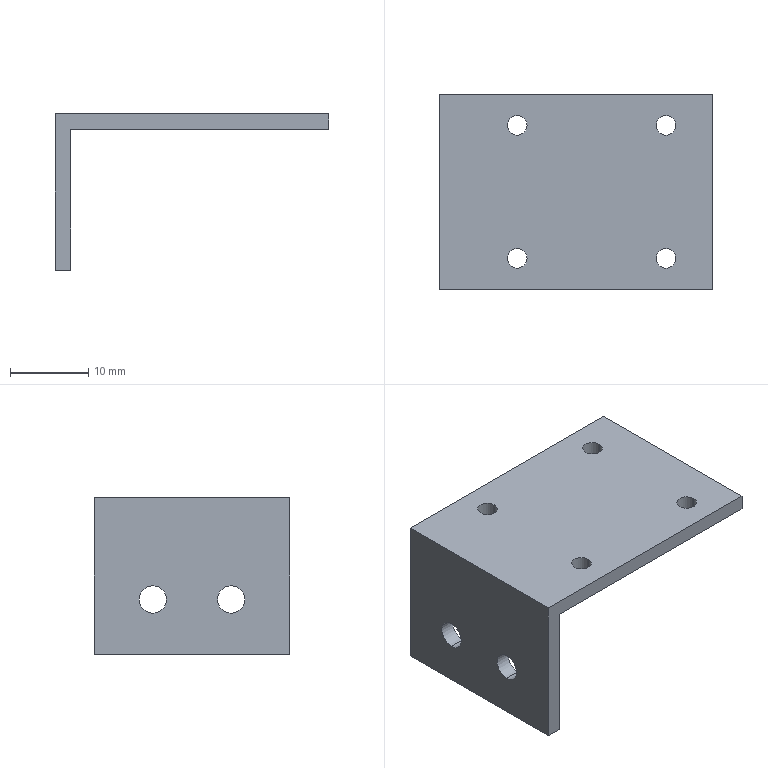Part | STEP file | 0244_220_Blacket | 1 solid | 20 faces | box 35 x 25 x 20 mm | volume 2572 mm3 | cylinder 12 | plane 8 | commonest cylinder face diameters 2.5 x8 3.5 x4